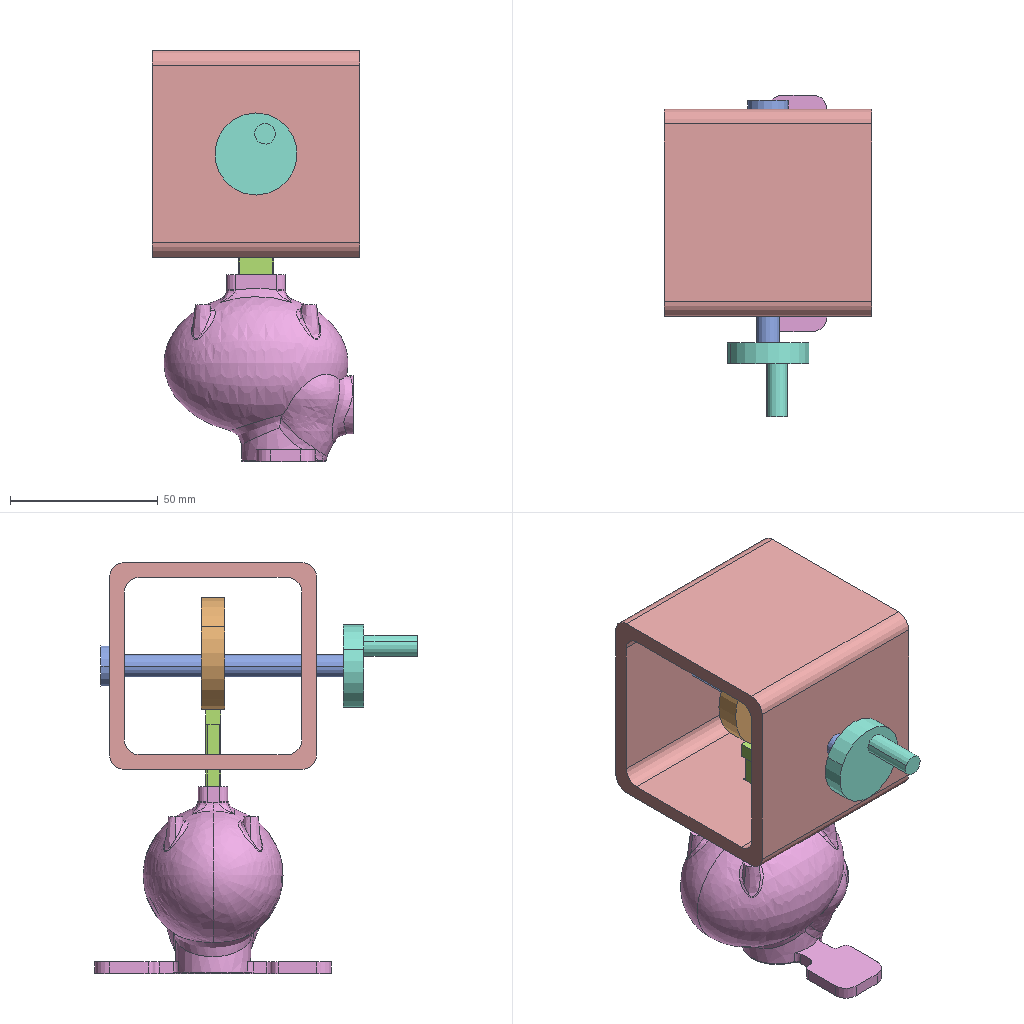Assembly | SolidWorks | 6 different items | 6 placed | box 70 x 109 x 139 mm
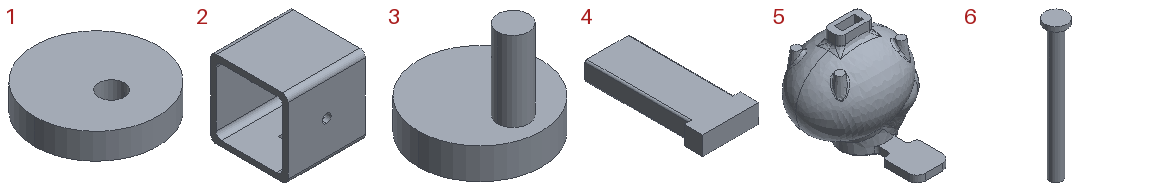Parts list (item | quantity | size | volume | features):
1 | x1 | 38 x 38 x 8 mm | 8691 mm3 | features Extrusion 1
2 | x1 | 70 x 70 x 70 mm | 90163 mm3 | features Cut 3, Extrusion 1, Fillet 1
3 | x1 | 27.8 x 27.8 x 25 mm | 4655 mm3 | features Cut 1, Extrusion 1, ICE 1
4 | x1 | 15 x 33 x 5 mm | 2049 mm3 | features Extrusion 1, Fillet 1, ICE 1
5 | x1 | 63.97 x 80 x 63.184 mm | 89467 mm3 | features Fillet 4, ICE 2, BaseBody 1, BossThin 1, Cut 1, MirrorPattern 1
6 | x1 | 13.8 x 13.8 x 88 mm | 4510 mm3 | features Extrusion 1, ICE 1
Mates (type | each side: item.copy, entity, surface, feature):
InPlace | 6.1 plane | assembly plane
InPlace | assembly plane | assembly plane | 2 times
Concentric | 2.1 face cylinder Cut-Extrude3 | assembly face
Concentric | 6.1 face cylinder Boss-Extrude1 | assembly face
Width | 2.1 face plane Cut-Extrude1 | 2.1 face plane Cut-Extrude1 | assembly face | assembly face
Width | 2.1 face plane Cut-Extrude2 | 2.1 face plane Cut-Extrude2 | 4.1 face plane Boss-Extrude1 | 4.1 face plane Boss-Extrude1
Width | 2.1 face plane Cut-Extrude2 | 2.1 face plane Cut-Extrude2 | 4.1 face plane Boss-Extrude2 | 4.1 face plane Boss-Extrude2
Tangent | assembly face | 4.1 face plane Boss-Extrude1
Parallel | 2.1 face plane Boss-Extrude1 | 4.1 face plane Boss-Extrude2
Coincident | 4.1 face plane Boss-Extrude2 | 5.1 face plane Cut-Extrude1
Width | 5.1 face plane Boss-Extrude1 | 5.1 face plane Boss-Extrude1 | 4.1 face plane Boss-Extrude1 | 4.1 face plane Boss-Extrude1
Width | 5.1 face plane Boss-Extrude1 | 5.1 face plane Boss-Extrude1 | 4.1 face plane Boss-Extrude2 | 4.1 face plane Boss-Extrude2
Coincident | 2.1 plane | assembly plane | 2 times
InPlace | 6.1 face plane Boss-Extrude1 | assembly plane
Concentric | 6.1 face cylinder Boss-Extrude1 | 3.1 face cylinder Cut-Extrude1
Coincident | 6.1 face plane Boss-Extrude1 | 3.1 face plane Cut-Extrude1
Parallel | 6.1 face cylinder Boss-Extrude1 | 3.1 face cylinder Boss-Extrude2
Concentric | 2.1 face cylinder Cut-Extrude3 | 6.1 face cylinder Boss-Extrude1
Parallel | assembly select_type:0 | 3.1 select_type:24
Concentric | 6.1 face cylinder Boss-Extrude1 | 1.1 face cylinder Boss-Extrude1
Width | 1.1 face plane Boss-Extrude1 | 1.1 face plane Boss-Extrude1 | 4.1 face plane Boss-Extrude1 | 4.1 face plane Boss-Extrude1
Tangent | 4.1 face plane Boss-Extrude1 | 1.1 face cylinder Boss-Extrude1
Parallel | 3.1 select_type:24 | 1.1 select_type:24